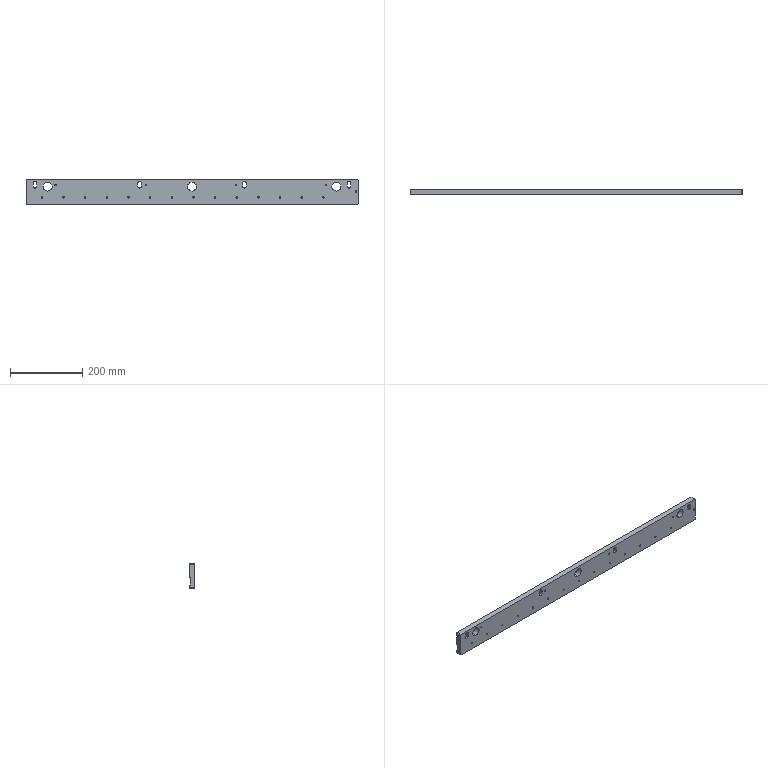Part | NX | features BREP 1 | 1 solid | 102 faces | box 920 x 15 x 70 mm | volume 888943 mm3 | cylinder 68 | plane 34 | commonest cylinder face diameters 4.2 x38 10 x12 15 x12 25 x6